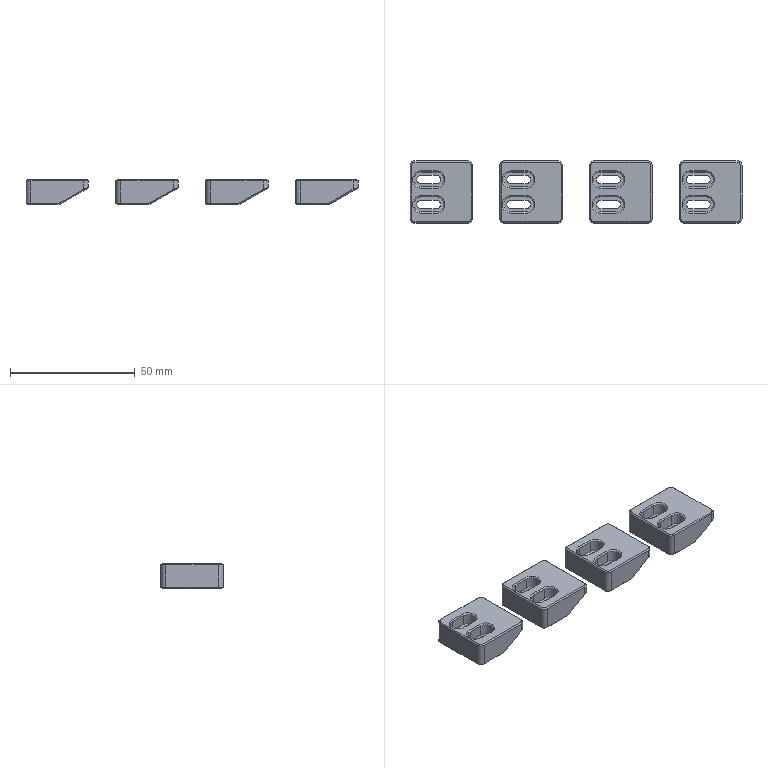NC program | NX | posted with a generic post | part box 133 x 25 x 10 mm
Lines 19 to 886 of 9691:
(ZLEVEL_PROFILE , TOOL : D10)
N36 T15 M6
N38 G54
N40 G17 G0 G90 X36.47 Y5.92 S9500 M3
N42 G43 Z30. H15
N44 Z1.5
N46 G94 G1 Y11.15 Z1.226 F2500.
N48 X36.806 Y12.743 Z1.141
N50 X37.497 Y14.216 Z1.055
N52 X38.508 Y15.492 Z0.97
N54 X39.784 Y16.503 Z0.885
N56 X41.257 Y17.194 Z0.799
N58 X42.85 Y17.53 Z0.714
N60 X54.23 Z0.118
N62 X54.954 Y17.514 Z0.08
N64 X56.387 Y17.24 Z0.003
N66 X57.755 Y16.733 Z-0.073
N68 X58.86 Y16.098 Z-0.14
N70 X59.864 Y15.126 Z-0.213
N72 X60.565 Y13.916 Z-0.287
N74 X60.907 Y12.56 Z-0.36
N76 Y12.01 Z-0.389
N78 Y-12.
N80 G2 X58.347 Y-16.392 R5.046
N82 X54.23 Y-17.53 R8.796
N84 G1 X43.5
N86 G2 X36.47 Y-10.5 R7.03
N88 G1 Y10.5
N90 G2 X43.5 Y17.53 R7.03
N92 G1 X54.23
N94 G2 X58.383 Y16.372 R8.727
N96 X60.907 Y12.01 R5.031
N98 G1 X61.623 Y-11.663 Z-0.802
N100 X61.634 Y-12.076 Z-0.808
N102 X61.622 Y-12.488 Z-0.815
N104 X61.572 Y-12.922 Z-0.822
N106 X61.484 Y-13.351 Z-0.828
N108 X61.358 Y-13.769 Z-0.835
N110 X61.195 Y-14.174 Z-0.842
N112 X60.999 Y-14.561 Z-0.848
N114 X60.767 Y-14.93 Z-0.855
N116 X60.508 Y-15.273 Z-0.862
N118 X60.214 Y-15.591 Z-0.868
N120 X59.9 Y-15.878 Z-0.875
N122 X59.583 Y-16.161 Z-0.882
N124 G2 X58.939 Y-16.543 R5.086
N126 G1 X57.939 Y-17.043
N128 G2 X55.562 Y-17.6 R5.314
N130 G1 X43.5
N132 G2 X36.41 Y-10.824 R7.1
N134 X36.4 Y-10.5 R5.1
N136 G1 Y10.5
N138 G2 X43.185 Y17.59 R7.1
N140 X43.5 Y17.6 R5.1
N142 G1 X55.562
N144 G2 X57.939 Y17.043 R5.314
N146 G1 X58.939 Y16.543
N148 G2 X61.761 Y12.014 R5.086
N150 G1 X61.773 Y11.627 Z-0.889
N152 X62.487 Y-11.986 Z-1.301
N154 X62.48 Y-12.429 Z-1.307
N156 X62.432 Y-12.868 Z-1.314
N158 X62.35 Y-13.303 Z-1.321
N160 X62.216 Y-13.726 Z-1.328
N162 X62.15 Y-13.936 Z-1.331
N164 X62.066 Y-14.14 Z-1.334
N166 X61.973 Y-14.339 Z-1.338
N168 X61.845 Y-14.525 Z-1.341
N170 X61.755 Y-14.725 Z-1.345
N172 X61.637 Y-14.909 Z-1.348
N174 X61.51 Y-15.088 Z-1.351
N176 X61.371 Y-15.259 Z-1.355
N178 X61.081 Y-15.58 Z-1.362
N180 X60.772 Y-15.886 Z-1.368
N182 X60.44 Y-16.156 Z-1.375
N184 X60.081 Y-16.395 Z-1.382
N186 G2 X59.805 Y-16.543 R5.086
N188 G1 X58.805 Y-17.043
N190 G2 X56.428 Y-17.6 R5.641
N192 G1 X43.5
N194 G2 X36.4 Y-10.5 R7.1
N196 G1 Y10.5
N198 G2 X43.5 Y17.6 R7.1
N200 G1 X56.428
N202 G2 X58.805 Y17.043 R5.314
N204 G1 X59.805 Y16.543
N206 G2 X62.627 Y12.02 R5.086
N208 G1 X62.639 Y11.632 Z-1.389
N210 X63.353 Y-11.98 Z-1.801
N212 X63.347 Y-12.423 Z-1.807
N214 X63.299 Y-12.862 Z-1.814
N216 X63.218 Y-13.297 Z-1.821
N218 X63.084 Y-13.72 Z-1.828
N220 X63.018 Y-13.931 Z-1.831
N222 X62.935 Y-14.134 Z-1.834
N224 X62.842 Y-14.334 Z-1.838
N226 X62.715 Y-14.52 Z-1.841
N228 X62.625 Y-14.72 Z-1.845
N230 X62.507 Y-14.904 Z-1.848
N232 X62.38 Y-15.083 Z-1.851
N234 X62.241 Y-15.254 Z-1.855
N236 X61.952 Y-15.576 Z-1.862
N238 X61.642 Y-15.882 Z-1.868
N240 X61.311 Y-16.152 Z-1.875
N242 X60.952 Y-16.392 Z-1.882
N244 G2 X60.671 Y-16.543 R5.086
N246 G1 X59.671 Y-17.043
N248 G2 X57.294 Y-17.6 R5.717
N250 G1 X43.5
N252 G2 X36.4 Y-10.5 R7.1
N254 G1 Y10.5
N256 G2 X43.5 Y17.6 R7.1
N258 G1 X57.294
N260 G2 X59.671 Y17.043 R5.314
N262 G1 X60.671 Y16.543
N264 G2 X63.493 Y12.026 R5.086
N266 G1 X63.505 Y11.639 Z-1.889
N268 X64.219 Y-11.974 Z-2.301
N270 X64.214 Y-12.416 Z-2.307
N272 X64.167 Y-12.855 Z-2.314
N274 X64.085 Y-13.29 Z-2.321
N276 X63.953 Y-13.713 Z-2.328
N278 X63.887 Y-13.924 Z-2.331
N280 X63.804 Y-14.127 Z-2.334
N282 X63.711 Y-14.327 Z-2.338
N284 X63.584 Y-14.513 Z-2.341
N286 X63.495 Y-14.714 Z-2.345
N288 X63.377 Y-14.898 Z-2.348
N290 X63.251 Y-15.077 Z-2.351
N292 X63.112 Y-15.249 Z-2.355
N294 X62.823 Y-15.571 Z-2.362
N296 X62.514 Y-15.878 Z-2.368
N298 X62.183 Y-16.148 Z-2.375
N300 X61.825 Y-16.388 Z-2.382
N302 G2 X61.537 Y-16.543 R5.086
N304 G1 X60.537 Y-17.043
N306 G2 X58.16 Y-17.6 R5.75
N308 G1 X43.5
N310 G2 X36.4 Y-10.5 R7.1
N312 G1 Y10.5
N314 G2 X43.5 Y17.6 R7.1
N316 G1 X58.16
N318 G2 X60.537 Y17.043 R5.314
N320 G1 X61.537 Y16.543
N322 G2 X64.359 Y12.034 R5.086
N324 G1 X64.371 Y11.647 Z-2.389
N326 X65.085 Y-11.966 Z-2.801
N328 X65.08 Y-12.408 Z-2.807
N330 X65.034 Y-12.846 Z-2.814
N332 X64.954 Y-13.281 Z-2.821
N334 X64.822 Y-13.705 Z-2.828
N336 X64.757 Y-13.916 Z-2.831
N338 X64.674 Y-14.119 Z-2.834
N340 X64.581 Y-14.319 Z-2.838
N342 X64.455 Y-14.506 Z-2.841
N344 X64.366 Y-14.706 Z-2.845
N346 X64.248 Y-14.891 Z-2.848
N348 X64.122 Y-15.07 Z-2.851
N350 X63.984 Y-15.242 Z-2.855
N352 X63.695 Y-15.565 Z-2.862
N354 X63.387 Y-15.872 Z-2.868
N356 X63.056 Y-16.143 Z-2.875
N358 X62.698 Y-16.384 Z-2.882
N360 G2 X62.403 Y-16.543 R5.086
N362 G1 X61.403 Y-17.043
N364 G2 X59.026 Y-17.6 R5.314
N366 G1 X43.5
N368 G2 X36.4 Y-10.5 R7.1
N370 G1 Y10.5
N372 G2 X43.5 Y17.6 R7.1
N374 G1 X59.026
N376 G2 X61.403 Y17.043 R5.314
N378 G1 X62.403 Y16.543
N380 G2 X65.225 Y12.043 R5.086
N382 G1 X65.237 Y11.656 Z-2.889
N384 X65.951 Y-11.957 Z-3.301
N386 X65.947 Y-12.398 Z-3.307
N388 X65.902 Y-12.836 Z-3.314
N390 X65.823 Y-13.271 Z-3.321
N392 X65.692 Y-13.695 Z-3.328
N394 X65.627 Y-13.906 Z-3.331
N396 X65.544 Y-14.11 Z-3.334
N398 X65.452 Y-14.31 Z-3.338
N400 X65.327 Y-14.497 Z-3.341
N402 X65.238 Y-14.697 Z-3.345
N404 X65.121 Y-14.882 Z-3.348
N406 X64.995 Y-15.062 Z-3.351
N408 X64.857 Y-15.234 Z-3.355
N410 X64.569 Y-15.558 Z-3.362
N412 X64.261 Y-15.865 Z-3.368
N414 X63.931 Y-16.137 Z-3.375
N416 X63.573 Y-16.379 Z-3.382
N418 G2 X63.269 Y-16.543 R5.086
N420 G1 X62.269 Y-17.043
N422 G2 X59.892 Y-17.6 R5.314
N424 G1 X43.5
N426 G2 X36.4 Y-10.5 R7.1
N428 G1 Y10.5
N430 G2 X43.5 Y17.6 R7.1
N432 G1 X59.892
N434 G2 X62.269 Y17.043 R5.314
N436 G1 X63.269 Y16.543
N438 G2 X66.091 Y12.055 R5.086
N440 G1 X66.103 Y11.667 Z-3.389
N442 X66.162 Y9.732 Z-3.422
N444 X66.817 Y-11.945 Z-3.801
N446 X66.814 Y-12.386 Z-3.807
N448 X66.77 Y-12.823 Z-3.814
N450 X66.692 Y-13.259 Z-3.821
N452 X66.563 Y-13.683 Z-3.828
N454 X66.498 Y-13.894 Z-3.831
N456 X66.416 Y-14.098 Z-3.834
N458 X66.324 Y-14.298 Z-3.838
N460 X66.199 Y-14.486 Z-3.841
N462 X66.111 Y-14.687 Z-3.845
N464 X65.994 Y-14.871 Z-3.848
N466 X65.869 Y-15.051 Z-3.851
N468 X65.731 Y-15.224 Z-3.855
N470 X65.444 Y-15.549 Z-3.862
N472 X65.137 Y-15.857 Z-3.868
N474 X64.807 Y-16.13 Z-3.875
N476 X64.45 Y-16.372 Z-3.882
N478 G2 X64.135 Y-16.543 R5.086
N480 G1 X63.135 Y-17.043
N482 G2 X60.758 Y-17.6 R5.314
N484 G1 X43.5
N486 G2 X36.4 Y-10.5 R7.1
N488 G1 Y10.5
N490 G2 X43.5 Y17.6 R7.1
N492 G1 X60.758
N494 G2 X63.135 Y17.043 R5.314
N496 G1 X64.135 Y16.543
N498 G2 X66.957 Y12.068 R5.086
N500 G1 X66.969 Y11.681 Z-3.889
N502 X66.981 Y11.294 Z-3.895
N504 X67.683 Y-11.932 Z-4.301
N506 X67.681 Y-12.371 Z-4.307
N508 X67.639 Y-12.807 Z-4.314
N510 X67.562 Y-13.243 Z-4.321
N512 X67.434 Y-13.668 Z-4.328
N514 X67.37 Y-13.879 Z-4.331
N516 X67.288 Y-14.084 Z-4.334
N518 X67.197 Y-14.284 Z-4.338
N520 X67.073 Y-14.472 Z-4.341
N522 X66.985 Y-14.673 Z-4.345
N524 X66.869 Y-14.859 Z-4.348
N526 X66.744 Y-15.039 Z-4.351
N528 X66.607 Y-15.212 Z-4.355
N530 X66.321 Y-15.538 Z-4.362
N532 X66.014 Y-15.847 Z-4.368
N534 X65.686 Y-16.121 Z-4.375
N536 X65.329 Y-16.365 Z-4.382
N538 G2 X65.001 Y-16.543 R5.086
N540 G1 X64.001 Y-17.043
N542 G2 X61.624 Y-17.6 R5.314
N544 G1 X43.5
N546 G2 X36.4 Y-10.5 R7.1
N548 G1 Y10.5
N550 G2 X43.5 Y17.6 R7.1
N552 G1 X61.624
N554 G2 X64.001 Y17.043 R5.314
N556 G1 X65.001 Y16.543
N558 G2 X67.823 Y12.085 R5.086
N560 G1 X67.835 Y11.698 Z-4.389
N562 X67.847 Y11.31 Z-4.395
N564 X68.549 Y-11.915 Z-4.801
N566 Y-12.353 Z-4.807
N568 X68.508 Y-12.789 Z-4.814
N570 X68.432 Y-13.225 Z-4.821
N572 X68.306 Y-13.65 Z-4.828
N574 X68.243 Y-13.862 Z-4.831
N576 X68.162 Y-14.066 Z-4.834
N578 X68.072 Y-14.268 Z-4.838
N580 X67.949 Y-14.456 Z-4.841
N582 X67.861 Y-14.658 Z-4.845
N584 X67.746 Y-14.843 Z-4.848
N586 X67.622 Y-15.024 Z-4.851
N588 X67.485 Y-15.198 Z-4.855
N590 X67.2 Y-15.525 Z-4.862
N592 X66.894 Y-15.835 Z-4.868
N594 X66.567 Y-16.111 Z-4.875
N596 X66.211 Y-16.355 Z-4.882
N598 G2 X65.867 Y-16.543 R5.086
N600 G1 X64.867 Y-17.043
N602 G2 X62.49 Y-17.6 R5.314
N604 G1 X43.5
N606 G2 X36.4 Y-10.5 R7.1
N608 G1 Y10.5
N610 G2 X43.5 Y17.6 R7.1
N612 G1 X62.49
N614 G2 X64.867 Y17.043 R5.314
N616 G1 X65.867 Y16.543
N618 G2 X68.688 Y12.105 R5.086
N620 G1 X68.701 Y11.717 Z-4.889
N622 X68.713 Y11.33 Z-4.895
N624 X69.415 Y-11.895 Z-5.301
N626 X69.416 Y-12.332 Z-5.307
N628 X69.38 Y-12.767 Z-5.314
N630 X69.305 Y-13.204 Z-5.321
N632 X69.19 Y-13.632 Z-5.328
N634 X69.04 Y-14.048 Z-5.334
N636 X68.851 Y-14.448 Z-5.341
N638 X68.632 Y-14.828 Z-5.348
N640 X68.377 Y-15.188 Z-5.355
N642 X68.095 Y-15.519 Z-5.362
N644 X67.783 Y-15.826 Z-5.368
N646 X67.452 Y-16.098 Z-5.375
N648 X67.096 Y-16.344 Z-5.382
N650 G2 X66.733 Y-16.543 R5.086
N652 G1 X65.733 Y-17.043
N654 G2 X63.356 Y-17.6 R5.596
N656 G1 X43.5
N658 G2 X36.4 Y-10.5 R7.1
N660 G1 Y10.5
N662 G2 X43.5 Y17.6 R7.1
N664 G1 X63.356
N666 G2 X65.733 Y17.043 R5.314
N668 G1 X66.733 Y16.543
N670 G2 X69.554 Y12.128 R5.086
N672 G1 X69.567 Y11.741 Z-5.389
N674 X69.579 Y11.354 Z-5.395
N676 X70.281 Y-11.871 Z-5.801
N678 X70.277 Y-12.305 Z-5.807
N680 X70.227 Y-12.737 Z-5.814
N682 X70.15 Y-13.17 Z-5.821
N684 X70.02 Y-13.593 Z-5.828
N686 X69.958 Y-13.803 Z-5.831
N688 X69.874 Y-14.005 Z-5.834
N690 X69.782 Y-14.205 Z-5.838
N692 X69.667 Y-14.395 Z-5.841
N694 X69.452 Y-14.771 Z-5.848
N696 X69.192 Y-15.122 Z-5.855
N698 X68.907 Y-15.443 Z-5.862
N700 X68.602 Y-15.748 Z-5.868
N702 X68.281 Y-16.022 Z-5.875
N704 X67.944 Y-16.281 Z-5.882
N706 G2 X67.052 Y-16.816 R6.754
N708 G1 X66.599 Y-17.043
N710 G2 X64.222 Y-17.6 R5.314
N712 G1 X43.5
N714 G2 X36.4 Y-10.5 R7.1
N716 G1 Y10.5
N718 G2 X43.5 Y17.6 R7.1
N720 G1 X64.222
N722 G2 X66.599 Y17.043 R5.626
N724 G1 X67.08 Y16.803
N726 G2 X69.365 Y14.946 R6.784
N728 X70.414 Y12.176 R4.895
N730 G1 X70.433 Y11.798 Z-5.888
N732 X70.445 Y11.421 Z-5.895
N734 X71.118 Y-10.842 Z-6.284
N736 X71.128 Y-11.219 Z-6.29
N738 X71.119 Y-11.603 Z-6.297
N740 X71.079 Y-11.987 Z-6.303
N742 X70.981 Y-12.403 Z-6.31
N744 X70.882 Y-12.818 Z-6.316
N746 X70.742 Y-13.21 Z-6.323
N748 X70.586 Y-13.599 Z-6.33
N750 X70.408 Y-13.968 Z-6.336
N752 X70.207 Y-14.327 Z-6.343
N754 X69.991 Y-14.67 Z-6.349
N756 X69.758 Y-15.003 Z-6.356
N758 X69.511 Y-15.315 Z-6.363
N760 X69.249 Y-15.614 Z-6.369
N762 X68.974 Y-15.901 Z-6.376
N764 X68.679 Y-16.168 Z-6.382
N766 X68.612 Y-16.225
N768 G2 X67.451 Y-16.958 R5.136
N770 X64.5 Y-17.6 R7.1
N772 G1 X43.5
N774 G2 X36.4 Y-10.5 R7.1
N776 G1 Y10.5
N778 G2 X43.5 Y17.6 R7.1
N780 G1 X64.5
N782 G2 X67.315 Y17.018 R7.1
N784 X70.254 Y14.296 R6.786
N786 G1 X70.469 Y13.916
N788 G2 X71.069 Y12.341 R7.238
N790 G1 X71.162 Y11.968 Z-6.389
N792 X71.235 Y11.591 Z-6.396
N794 X71.275 Y11.209 Z-6.402
N796 X71.312 Y10.826 Z-6.409
N798 X71.33 Y10.442 Z-6.416
N800 X71.335 Y10.058 Z-6.423
N802 X71.339 Y9.674 Z-6.429
N804 X71.536 Y-9.89 Z-6.771
N806 X71.54 Y-10.277 Z-6.777
N808 X71.536 Y-10.663 Z-6.784
N810 X71.522 Y-11.059 Z-6.791
N812 X71.485 Y-11.454 Z-6.798
N814 X71.429 Y-11.847 Z-6.804
N816 X71.352 Y-12.236 Z-6.811
N818 X71.257 Y-12.622 Z-6.818
N820 X71.14 Y-13.001 Z-6.824
N822 X70.994 Y-13.37 Z-6.831
N824 X70.823 Y-13.729 Z-6.838
N826 X70.634 Y-14.075 Z-6.844
N828 X70.425 Y-14.412 Z-6.851
N830 X70.199 Y-14.734 Z-6.858
N832 X69.956 Y-15.044 Z-6.864
N834 X69.697 Y-15.337 Z-6.871
N836 X69.422 Y-15.617 Z-6.878
N838 X69.135 Y-15.879 Z-6.885
N840 X68.832 Y-16.125 Z-6.891
N842 X68.52 Y-16.352 Z-6.898
N844 X68.194 Y-16.563 Z-6.905
N846 X67.861 Y-16.754 Z-6.911
N848 X67.518 Y-16.927 Z-6.918
N850 X67.166 Y-17.08 Z-6.925
N852 X66.807 Y-17.215 Z-6.931
N854 X66.441 Y-17.33 Z-6.938
N856 X66.069 Y-17.424 Z-6.945
N858 X65.693 Y-17.499 Z-6.952
N860 X65.313 Y-17.553 Z-6.958
N862 X64.931 Y-17.587 Z-6.965
N864 X64.548 Y-17.6 Z-6.972
N866 X64.164 Z-6.978
N868 X49.971 Z-7.226
N870 X43.5
N872 G2 X36.4 Y-10.5 R7.1
N874 G1 Y10.5
N876 G2 X43.5 Y17.6 R7.1
N878 G1 X64.5
N880 G2 X71.337 Y12.416 R7.1
N882 G1 X71.431 Y12.041 Z-7.233
N884 X71.504 Y11.661 Z-7.24
N886 X71.557 Y11.277 Z-7.246
N888 X71.589 Y10.891 Z-7.253
N890 X71.6 Y10.505 Z-7.26
N892 Y10.118 Z-7.267
N894 Y-10.011 Z-7.618
N896 Y-10.399 Z-7.625
N898 X71.594 Y-10.786 Z-7.631
N900 X71.568 Y-11.172 Z-7.638
N902 X71.521 Y-11.556 Z-7.645
N904 X71.453 Y-11.937 Z-7.652
N906 X71.364 Y-12.314 Z-7.658
N908 X71.255 Y-12.685 Z-7.665
N910 X71.126 Y-13.05 Z-7.672
N912 X70.978 Y-13.407 Z-7.679
N914 X70.809 Y-13.756 Z-7.686
N916 X70.623 Y-14.095 Z-7.692
N918 X70.418 Y-14.423 Z-7.699
N920 X70.195 Y-14.74 Z-7.706
N922 X69.956 Y-15.044 Z-7.713
N924 X69.7 Y-15.334 Z-7.719
N926 X69.429 Y-15.611 Z-7.726
N928 X69.143 Y-15.872 Z-7.733
N930 X68.843 Y-16.117 Z-7.74
N932 X68.531 Y-16.345 Z-7.746
N934 X68.206 Y-16.556 Z-7.753
N936 X67.871 Y-16.749 Z-7.76
N938 X67.525 Y-16.923 Z-7.767
N940 X67.171 Y-17.079 Z-7.773
N942 X66.808 Y-17.214 Z-7.78
N944 X66.439 Y-17.33 Z-7.787
N946 X66.064 Y-17.426 Z-7.794
N948 X65.684 Y-17.501 Z-7.8
N950 X65.301 Y-17.555 Z-7.807
N952 X64.915 Y-17.588 Z-7.814
N954 X64.528 Y-17.6 Z-7.821
N956 X64.141 Z-7.827
N958 X43.625 Z-8.186
N960 X43.238 Y-17.595 Z-8.192
N962 X42.852 Y-17.57 Z-8.199
N964 X42.468 Y-17.525 Z-8.206
N966 X42.086 Y-17.458 Z-8.213
N968 X41.709 Y-17.371 Z-8.219
N970 X41.338 Y-17.263 Z-8.226
N972 G2 X36.4 Y-10.5 R7.1
N974 G1 Y10.5
N976 G2 X43.5 Y17.6 R7.1
N978 G1 X64.5
N980 G2 X71.337 Y12.416 R7.1
N982 G1 X71.43 Y12.043 Z-8.233
N984 X71.504 Y11.665 Z-8.239
N986 X71.557 Y11.284 Z-8.246
N988 X71.589 Y10.9 Z-8.253
N990 X71.6 Y10.515 Z-8.26
N992 Y10.13 Z-8.266
N994 Y-9.888 Z-8.616
N996 Y-10.273 Z-8.622
N998 X71.598 Y-10.658 Z-8.629
N1000 X71.579 Y-11.042 Z-8.636
N1002 X71.54 Y-11.425 Z-8.643
N1004 X71.479 Y-11.805 Z-8.649
N1006 X71.398 Y-12.181 Z-8.656
N1008 X71.297 Y-12.553 Z-8.663
N1010 X71.176 Y-12.918 Z-8.67
N1012 X71.035 Y-13.276 Z-8.676
N1014 X70.875 Y-13.626 Z-8.683
N1016 X70.696 Y-13.967 Z-8.69
N1018 X70.499 Y-14.298 Z-8.696
N1020 X70.284 Y-14.617 Z-8.703
N1022 X70.053 Y-14.925 Z-8.71
N1024 X69.805 Y-15.219 Z-8.717
N1026 X69.541 Y-15.5 Z-8.723
N1028 X69.263 Y-15.766 Z-8.73
N1030 X68.97 Y-16.016 Z-8.737
N1032 X68.665 Y-16.25 Z-8.743
N1034 X68.347 Y-16.467 Z-8.75
N1036 X68.018 Y-16.667 Z-8.757
N1038 X67.679 Y-16.849 Z-8.764
N1040 X67.33 Y-17.012 Z-8.77
N1042 X66.973 Y-17.155 Z-8.777
N1044 X66.609 Y-17.28 Z-8.784
N1046 X66.238 Y-17.384 Z-8.79
N1048 X65.863 Y-17.468 Z-8.797
N1050 X65.483 Y-17.532 Z-8.804
N1052 X65.1 Y-17.575 Z-8.811
N1054 X64.716 Y-17.597 Z-8.817
N1056 X64.331 Y-17.6 Z-8.824
N1058 X63.946 Z-8.831
N1060 X47.778 Z-9.113
N1062 X43.5
N1064 G2 X36.4 Y-10.5 R7.1
N1066 G1 Y10.5
N1068 G2 X43.5 Y17.6 R7.1
N1070 G1 X64.5
N1072 G2 X71.337 Y12.416 R7.1
N1074 G1 X71.43 Y12.043 Z-9.12
N1076 X71.504 Y11.665 Z-9.126
N1078 X71.557 Y11.284 Z-9.133
N1080 X71.589 Y10.9 Z-9.14
N1082 X71.6 Y10.515 Z-9.147
N1084 Y10.13 Z-9.153
N1086 Y-9.888 Z-9.503
N1088 Y-10.273 Z-9.509
N1090 X71.598 Y-10.658 Z-9.516
N1092 X71.579 Y-11.042 Z-9.523
N1094 X71.54 Y-11.425 Z-9.53
N1096 X71.479 Y-11.805 Z-9.536
N1098 X71.398 Y-12.181 Z-9.543
N1100 X71.297 Y-12.553 Z-9.55
N1102 X71.176 Y-12.918 Z-9.557
N1104 X71.035 Y-13.276 Z-9.563
N1106 X70.875 Y-13.626 Z-9.57
N1108 X70.696 Y-13.967 Z-9.577
N1110 X70.499 Y-14.298 Z-9.583
N1112 X70.284 Y-14.617 Z-9.59
N1114 X70.053 Y-14.925 Z-9.597
N1116 X69.805 Y-15.219 Z-9.604
N1118 X69.541 Y-15.5 Z-9.61
N1120 X69.263 Y-15.766 Z-9.617
N1122 X68.97 Y-16.016 Z-9.624
N1124 X68.665 Y-16.25 Z-9.63
N1126 X68.347 Y-16.467 Z-9.637
N1128 X68.018 Y-16.667 Z-9.644
N1130 X67.679 Y-16.849 Z-9.651
N1132 X67.33 Y-17.012 Z-9.657
N1134 X66.973 Y-17.155 Z-9.664
N1136 X66.609 Y-17.28 Z-9.671
N1138 X66.238 Y-17.384 Z-9.677
N1140 X65.863 Y-17.468 Z-9.684
N1142 X65.483 Y-17.532 Z-9.691
N1144 X65.1 Y-17.575 Z-9.698
N1146 X64.716 Y-17.597 Z-9.704
N1148 X64.331 Y-17.6 Z-9.711
N1150 X63.946 Z-9.718
N1152 X47.778 Z-10.
N1154 X43.5
N1156 G2 X36.4 Y-10.5 R7.1
N1158 G1 Y10.5
N1160 G2 X43.5 Y17.6 R7.1
N1162 G1 X64.5
N1164 G2 X71.6 Y10.5 R7.1
N1166 G1 Y-10.5
N1168 G2 X64.5 Y-17.6 R7.1
N1170 G1 X47.778
N1172 Z-8.5
N1174 G0 Z30.
N1176 X0.47 Y5.923
N1178 Z1.5
N1180 G1 Y11.15 Z1.226
N1182 X0.806 Y12.743 Z1.141
N1184 X1.497 Y14.216 Z1.055
N1186 X2.508 Y15.492 Z0.97
N1188 X3.784 Y16.503 Z0.885
N1190 X5.257 Y17.194 Z0.8
N1192 X6.85 Y17.53 Z0.714
N1194 X18.23 Z0.118
N1196 X18.957 Y17.514 Z0.08
N1198 X20.39 Y17.241 Z0.003
N1200 X21.758 Y16.737 Z-0.073
N1202 X22.389 Y16.377 Z-0.111
N1204 X22.868 Y16.092 Z-0.14
N1206 X23.86 Y15.114 Z-0.213
N1208 X24.554 Y13.906 Z-0.286
N1210 X24.902 Y12.557 Z-0.359
N1212 X24.907 Y12. Z-0.389
N1214 Y-12.
N1216 G2 X22.389 Y-16.377 R5.147
N1218 X18.23 Y-17.53 R8.837
N1220 G1 X7.5
N1222 G2 X0.47 Y-10.5 R7.03
N1224 G1 Y10.5
N1226 G2 X7.5 Y17.53 R7.03
N1228 G1 X18.23
N1230 G2 X22.389 Y16.377 R8.793
N1232 X24.907 Y12. R5.147
N1234 G1 X25.623 Y-11.672 Z-0.802
N1236 X25.634 Y-12.089 Z-0.808
N1238 X25.621 Y-12.505 Z-0.815
N1240 X25.569 Y-12.939 Z-0.822
N1242 X25.479 Y-13.366 Z-0.828
N1244 X25.353 Y-13.783 Z-0.835
N1246 X25.188 Y-14.188 Z-0.842
N1248 X24.992 Y-14.574 Z-0.848
N1250 X24.758 Y-14.942 Z-0.855
N1252 X24.499 Y-15.284 Z-0.862
N1254 X24.203 Y-15.6 Z-0.868
N1256 X23.89 Y-15.887 Z-0.875
N1258 X23.572 Y-16.169 Z-0.882
N1260 G2 X22.939 Y-16.543 R5.086
N1262 G1 X21.939 Y-17.043
N1264 G2 X19.562 Y-17.6 R5.314
N1266 G1 X7.5
N1268 G2 X0.408 Y-10.842 R7.1
N1270 G1 X0.411
N1272 G2 X0.4 Y-10.5 R5.1
N1274 G1 Y10.5
N1276 G2 X7.144 Y17.591 R7.1
N1278 G1 Y17.588
N1280 G2 X7.5 Y17.6 R5.1
N1282 G1 X19.562
N1284 G2 X21.939 Y17.043 R5.314
N1286 G1 X22.939 Y16.543
N1288 G2 X25.762 Y12.002 R5.086
N1290 G1 X25.773 Y11.615 Z-0.889
N1292 X26.487 Y-11.997 Z-1.301
N1294 X26.479 Y-12.441 Z-1.307
N1296 X26.43 Y-12.882 Z-1.314
N1298 X26.346 Y-13.316 Z-1.321
N1300 X26.211 Y-13.739 Z-1.328
N1302 X26.145 Y-13.949 Z-1.331
N1304 X26.06 Y-14.152 Z-1.334
N1306 X25.967 Y-14.351 Z-1.338
N1308 X25.838 Y-14.536 Z-1.341
N1310 X25.748 Y-14.736 Z-1.345
N1312 X25.63 Y-14.92 Z-1.348
N1314 X25.502 Y-15.098 Z-1.351
N1316 X25.363 Y-15.269 Z-1.355
N1318 X25.072 Y-15.59 Z-1.362
N1320 X24.762 Y-15.894 Z-1.368
N1322 X24.43 Y-16.163 Z-1.375
N1324 X24.07 Y-16.401 Z-1.382
N1326 G2 X23.805 Y-16.543 R5.086
N1328 G1 X22.805 Y-17.043
N1330 G2 X20.428 Y-17.6 R5.314
N1332 G1 X7.5
N1334 G2 X0.4 Y-10.5 R7.1
N1336 G1 Y10.5
N1338 G2 X7.5 Y17.6 R7.1
N1340 G1 X20.428
N1342 G2 X22.805 Y17.043 R5.314
N1344 G1 X23.805 Y16.543
N1346 G2 X26.628 Y12.005 R5.086
N1348 G1 X26.639 Y11.618 Z-1.389
N1350 X27.353 Y-11.994 Z-1.801
N1352 X27.346 Y-12.438 Z-1.807
N1354 X27.296 Y-12.878 Z-1.814
N1356 X27.213 Y-13.313 Z-1.821
N1358 X27.079 Y-13.735 Z-1.828
N1360 X27.012 Y-13.946 Z-1.831
N1362 X26.928 Y-14.149 Z-1.834
N1364 X26.834 Y-14.348 Z-1.838
N1366 X26.706 Y-14.533 Z-1.841
N1368 X26.616 Y-14.734 Z-1.845
N1370 X26.498 Y-14.917 Z-1.848
N1372 X26.37 Y-15.095 Z-1.851
N1374 X26.231 Y-15.266 Z-1.855
N1376 X25.94 Y-15.587 Z-1.862
N1378 X25.63 Y-15.892 Z-1.868
N1380 X25.298 Y-16.161 Z-1.875
N1382 X24.939 Y-16.4 Z-1.882
N1384 G2 X24.671 Y-16.543 R5.086
N1386 G1 X23.671 Y-17.043
N1388 G2 X21.294 Y-17.6 R5.314
N1390 G1 X7.5
N1392 G2 X0.4 Y-10.5 R7.1
N1394 G1 Y10.5
N1396 G2 X7.5 Y17.6 R7.1
N1398 G1 X21.294
N1400 G2 X23.671 Y17.043 R5.314
N1402 G1 X24.671 Y16.543
N1404 G2 X27.494 Y12.009 R5.086
N1406 G1 X27.505 Y11.622 Z-1.889
N1408 X28.219 Y-11.991 Z-2.301
N1410 X28.212 Y-12.434 Z-2.307
N1412 X28.163 Y-12.874 Z-2.314
N1414 X28.08 Y-13.309 Z-2.321
N1416 X27.946 Y-13.732 Z-2.328
N1418 X27.88 Y-13.942 Z-2.331
N1420 X27.795 Y-14.145 Z-2.334
N1422 X27.702 Y-14.344 Z-2.338
N1424 X27.574 Y-14.53 Z-2.341
N1426 X27.484 Y-14.73 Z-2.345
N1428 X27.366 Y-14.914 Z-2.348
N1430 X27.239 Y-15.092 Z-2.351
N1432 X27.1 Y-15.263 Z-2.355
N1434 X26.809 Y-15.584 Z-2.362
N1436 X26.499 Y-15.89 Z-2.368
N1438 X26.168 Y-16.159 Z-2.375
N1440 X25.808 Y-16.398 Z-2.382
N1442 G2 X25.537 Y-16.543 R5.086
N1444 G1 X24.537 Y-17.043
N1446 G2 X22.16 Y-17.6 R5.314
N1448 G1 X7.5
N1450 G2 X0.4 Y-10.5 R7.1
N1452 G1 Y10.5
N1454 G2 X7.5 Y17.6 R7.1
N1456 G1 X22.16
N1458 G2 X24.537 Y17.043 R5.314
N1460 G1 X25.537 Y16.543
N1462 G2 X28.36 Y12.013 R5.086
N1464 G1 X28.371 Y11.626 Z-2.389
N1466 X29.085 Y-11.987 Z-2.801
N1468 X29.078 Y-12.43 Z-2.807
N1470 X29.03 Y-12.869 Z-2.814
N1472 X28.948 Y-13.304 Z-2.821
N1474 X28.814 Y-13.727 Z-2.828
N1476 X28.748 Y-13.937 Z-2.831
N1478 X28.664 Y-14.14 Z-2.834
N1480 X28.57 Y-14.34 Z-2.838
N1482 X28.443 Y-14.526 Z-2.841
N1484 X28.353 Y-14.726 Z-2.845
N1486 X28.235 Y-14.91 Z-2.848
N1488 X28.108 Y-15.088 Z-2.851
N1490 X27.969 Y-15.26 Z-2.855
N1492 X27.679 Y-15.581 Z-2.862
N1494 X27.369 Y-15.887 Z-2.868
N1496 X27.038 Y-16.156 Z-2.875
N1498 X26.678 Y-16.395 Z-2.882
N1500 G2 X26.403 Y-16.543 R5.086
N1502 G1 X25.403 Y-17.043
N1504 G2 X23.026 Y-17.6 R5.314
N1506 G1 X7.5
N1508 G2 X0.4 Y-10.5 R7.1
N1510 G1 Y10.5
N1512 G2 X7.5 Y17.6 R7.1
N1514 G1 X23.026
N1516 G2 X25.403 Y17.043 R5.314
N1518 G1 X26.403 Y16.543
N1520 G2 X29.226 Y12.018 R5.086
N1522 G1 X29.237 Y11.631 Z-2.889
N1524 X29.951 Y-11.981 Z-3.301
N1526 X29.945 Y-12.424 Z-3.307
N1528 X29.897 Y-12.864 Z-3.314
N1530 X29.815 Y-13.298 Z-3.321
N1532 X29.682 Y-13.721 Z-3.328
N1534 X29.616 Y-13.932 Z-3.331
N1536 X29.532 Y-14.135 Z-3.334
N1538 X29.439 Y-14.335 Z-3.338
N1540 X29.312 Y-14.521 Z-3.341
N1542 X29.222 Y-14.721 Z-3.345
N1544 X29.104 Y-14.905 Z-3.348
N1546 X28.978 Y-15.084 Z-3.351
N1548 X28.839 Y-15.255 Z-3.355
N1550 X28.549 Y-15.577 Z-3.362
N1552 X28.24 Y-15.883 Z-3.368
N1554 X27.908 Y-16.153 Z-3.375
N1556 X27.549 Y-16.392 Z-3.382
N1558 G2 X27.269 Y-16.543 R5.086
N1560 G1 X26.269 Y-17.043
N1562 G2 X23.892 Y-17.6 R5.314
N1564 G1 X7.5
N1566 G2 X0.4 Y-10.5 R7.1
N1568 G1 Y10.5
N1570 G2 X7.5 Y17.6 R7.1
N1572 G1 X23.892
N1574 G2 X26.269 Y17.043 R5.314
N1576 G1 X27.269 Y16.543
N1578 G2 X30.092 Y12.025 R5.086
N1580 G1 X30.103 Y11.638 Z-3.389
N1582 X30.817 Y-11.975 Z-3.801
N1584 X30.812 Y-12.417 Z-3.807
N1586 X30.764 Y-12.856 Z-3.814
N1588 X30.683 Y-13.292 Z-3.821
N1590 X30.551 Y-13.715 Z-3.828
N1592 X30.485 Y-13.925 Z-3.831
N1594 X30.401 Y-14.129 Z-3.834
N1596 X30.309 Y-14.328 Z-3.838
N1598 X30.182 Y-14.515 Z-3.841
N1600 X30.092 Y-14.715 Z-3.845
N1602 X29.974 Y-14.899 Z-3.848
N1604 X29.848 Y-15.078 Z-3.851
N1606 X29.709 Y-15.25 Z-3.855
N1608 X29.42 Y-15.572 Z-3.862
N1610 X29.111 Y-15.879 Z-3.868
N1612 X28.78 Y-16.149 Z-3.875
N1614 X28.422 Y-16.389 Z-3.882
N1616 G2 X28.135 Y-16.543 R5.086
N1618 G1 X27.135 Y-17.043
N1620 G2 X24.758 Y-17.6 R5.634
N1622 G1 X7.5
N1624 G2 X0.4 Y-10.5 R7.1
N1626 G1 Y10.5
N1628 G2 X7.5 Y17.6 R7.1
N1630 G1 X24.758
N1632 G2 X27.135 Y17.043 R5.314
N1634 G1 X28.135 Y16.543
N1636 G2 X30.958 Y12.032 R5.086
N1638 G1 X30.969 Y11.645 Z-3.889
N1640 X31.683 Y-11.968 Z-4.301
N1642 X31.678 Y-12.409 Z-4.307
N1644 X31.632 Y-12.848 Z-4.314
N1646 X31.551 Y-13.283 Z-4.321
N1648 X31.42 Y-13.707 Z-4.328
N1650 X31.354 Y-13.917 Z-4.331
N1652 X31.271 Y-14.121 Z-4.334
N1654 X31.179 Y-14.321 Z-4.338
N1656 X31.052 Y-14.507 Z-4.341
N1658 X30.963 Y-14.708 Z-4.345
N1660 X30.845 Y-14.892 Z-4.348
N1662 X30.719 Y-15.071 Z-4.351
N1664 X30.581 Y-15.243 Z-4.355
N1666 X30.292 Y-15.566 Z-4.362
N1668 X29.984 Y-15.873 Z-4.368
N1670 X29.653 Y-16.144 Z-4.375
N1672 X29.295 Y-16.385 Z-4.382
N1674 G2 X29.001 Y-16.543 R5.086
N1676 G1 X28.001 Y-17.043
N1678 G2 X25.624 Y-17.6 R5.706
N1680 G1 X7.5
N1682 G2 X0.4 Y-10.5 R7.1
N1684 G1 Y10.5
N1686 G2 X7.5 Y17.6 R7.1
N1688 G1 X25.624
N1690 G2 X28.001 Y17.043 R5.314
N1692 G1 X29.001 Y16.543
N1694 G2 X31.823 Y12.041 R5.086
N1696 G1 X31.835 Y11.654 Z-4.389
N1698 X32.549 Y-11.958 Z-4.801
N1700 X32.545 Y-12.4 Z-4.807
N1702 X32.5 Y-12.838 Z-4.814
N1704 X32.42 Y-13.273 Z-4.821
N1706 X32.289 Y-13.697 Z-4.828
N1708 X32.224 Y-13.908 Z-4.831
N1710 X32.141 Y-14.111 Z-4.834
N1712 X32.049 Y-14.312 Z-4.838
N1714 X31.924 Y-14.499 Z-4.841
N1716 X31.835 Y-14.699 Z-4.845
N1718 X31.717 Y-14.884 Z-4.848
N1720 X31.592 Y-15.063 Z-4.851
N1722 X31.454 Y-15.236 Z-4.855
N1724 X31.165 Y-15.559 Z-4.862
N1726 X30.857 Y-15.867 Z-4.868
N1728 X30.527 Y-16.139 Z-4.875
N1730 X30.169 Y-16.38 Z-4.882
N1732 G2 X29.867 Y-16.543 R5.086
N1734 G1 X28.867 Y-17.043
N1736 G2 X26.49 Y-17.6 R5.758
N1738 G1 X7.5
N1740 G2 X0.4 Y-10.5 R7.1
N1742 G1 Y10.5
N1744 G2 X7.5 Y17.6 R7.1
N1746 G1 X26.49
N1748 G2 X28.867 Y17.043 R5.314
N1750 G1 X29.867 Y16.543
N1752 G2 X32.689 Y12.052 R5.086
N1754 G1 X32.701 Y11.665 Z-4.889
N1756 X32.842 Y7.02 Z-4.97
N1758 X33.415 Y-11.948 Z-5.301
N1760 X33.412 Y-12.388 Z-5.307
N1762 X33.371 Y-12.826 Z-5.314
N1764 X33.29 Y-13.262 Z-5.321